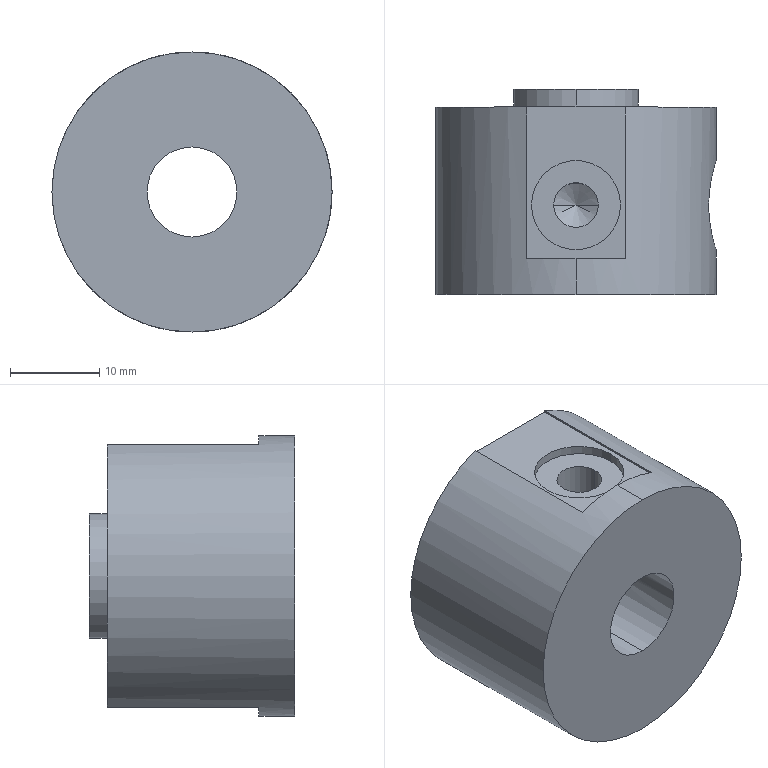Part | STEP file | 0229_Z_Cylinder_CG1BN25-50_2 | 1 solid | 54 faces | box 31.4 x 23 x 31.4 mm | volume 12893 mm3 | cylinder 26 | cone 14 | plane 14 | commonest cylinder face diameters 4.2 x8 10 x6 5 x4 6.8 x2 10.1 x2 14 x2